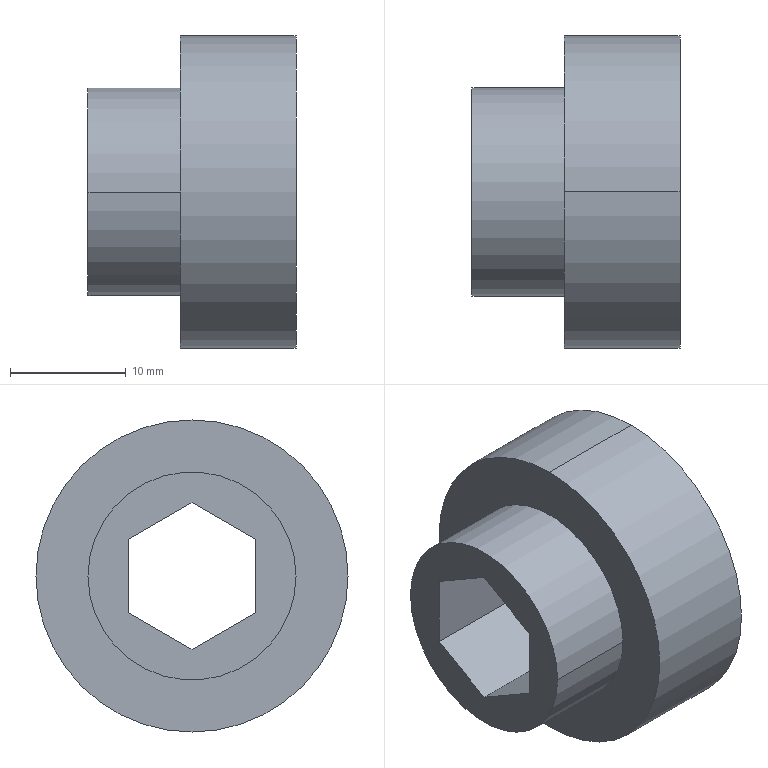Part | NX | features BREP 1 | 1 solid | 13 faces | box 18 x 27 x 27 mm | volume 5875 mm3 | plane 9 | cylinder 4 | commonest cylinder face diameters 18 x2 27 x2
STEP:
#1=CARTESIAN_POINT('',(-5.,0.,13.5));
#2=VERTEX_POINT('',#1);
#3=CARTESIAN_POINT('',(-5.,0.,-13.5));
#4=VERTEX_POINT('',#3);
#5=CARTESIAN_POINT('',(-5.,0.,0.));
#6=DIRECTION('',(1.,0.,0.));
#7=DIRECTION('',(0.,0.,1.));
#8=AXIS2_PLACEMENT_3D('',#5,#6,#7);
#9=CIRCLE('',#8,13.5);
#10=EDGE_CURVE('',#2,#4,#9,.T.);
#11=ORIENTED_EDGE('',*,*,#10,.F.);
#12=CARTESIAN_POINT('',(-5.,0.,0.));
#13=DIRECTION('',(1.,0.,0.));
#14=DIRECTION('',(0.,0.,-1.));
#15=AXIS2_PLACEMENT_3D('',#12,#13,#14);
#16=CIRCLE('',#15,13.5);
#17=EDGE_CURVE('',#4,#2,#16,.T.);
#18=ORIENTED_EDGE('',*,*,#17,.F.);
#19=EDGE_LOOP('',(#11,#18));
#20=FACE_BOUND('',#19,.T.);
#21=CARTESIAN_POINT('',(-5.,-9.,0.));
#22=VERTEX_POINT('',#21);
#23=CARTESIAN_POINT('',(-5.,9.,0.));
#24=VERTEX_POINT('',#23);
#25=CARTESIAN_POINT('',(-5.,0.,0.));
#26=DIRECTION('',(-1.,0.,0.));
#27=DIRECTION('',(0.,-1.,0.));
#28=AXIS2_PLACEMENT_3D('',#25,#26,#27);
#29=CIRCLE('',#28,9.);
#30=EDGE_CURVE('',#22,#24,#29,.T.);
#31=ORIENTED_EDGE('',*,*,#30,.F.);
#32=CARTESIAN_POINT('',(-5.,0.,0.));
#33=DIRECTION('',(-1.,0.,0.));
#34=DIRECTION('',(0.,1.,0.));
#35=AXIS2_PLACEMENT_3D('',#32,#33,#34);
#36=CIRCLE('',#35,9.);
#37=EDGE_CURVE('',#24,#22,#36,.T.);
#38=ORIENTED_EDGE('',*,*,#37,.F.);
#39=EDGE_LOOP('',(#31,#38));
#40=FACE_BOUND('',#39,.T.);
#41=CARTESIAN_POINT('',(-5.,0.,0.));
#42=DIRECTION('',(1.,0.,0.));
#43=DIRECTION('',(0.,1.,0.));
#44=AXIS2_PLACEMENT_3D('',#41,#42,#43);
#45=PLANE('',#44);
#46=ADVANCED_FACE('',(#20,#40),#45,.F.);
#47=CARTESIAN_POINT('',(5.,0.,13.5));
#48=VERTEX_POINT('',#47);
#49=CARTESIAN_POINT('',(-5.,0.,13.5));
#50=DIRECTION('',(1.,0.,0.));
#51=VECTOR('',#50,1000.);
#52=LINE('',#49,#51);
#53=EDGE_CURVE('',#48,#2,#52,.F.);
#54=ORIENTED_EDGE('',*,*,#53,.F.);
#55=CARTESIAN_POINT('',(5.,0.,-13.5));
#56=VERTEX_POINT('',#55);
#57=CARTESIAN_POINT('',(5.,0.,0.));
#58=DIRECTION('',(1.,0.,0.));
#59=DIRECTION('',(0.,0.,-1.));
#60=AXIS2_PLACEMENT_3D('',#57,#58,#59);
#61=CIRCLE('',#60,13.5);
#62=EDGE_CURVE('',#56,#48,#61,.T.);
#63=ORIENTED_EDGE('',*,*,#62,.F.);
#64=CARTESIAN_POINT('',(-5.,0.,-13.5));
#65=DIRECTION('',(1.,0.,0.));
#66=VECTOR('',#65,1000.);
#67=LINE('',#64,#66);
#68=EDGE_CURVE('',#56,#4,#67,.F.);
#69=ORIENTED_EDGE('',*,*,#68,.T.);
#70=ORIENTED_EDGE('',*,*,#17,.T.);
#71=EDGE_LOOP('',(#54,#63,#69,#70));
#72=FACE_BOUND('',#71,.T.);
#73=CARTESIAN_POINT('',(-5.,0.,0.));
#74=DIRECTION('',(1.,0.,0.));
#75=DIRECTION('',(0.,0.,-1.));
#76=AXIS2_PLACEMENT_3D('',#73,#74,#75);
#77=CYLINDRICAL_SURFACE('',#76,13.5);
#78=ADVANCED_FACE('',(#72),#77,.T.);
#79=ORIENTED_EDGE('',*,*,#68,.F.);
#80=CARTESIAN_POINT('',(5.,0.,0.));
#81=DIRECTION('',(1.,0.,0.));
#82=DIRECTION('',(0.,0.,1.));
#83=AXIS2_PLACEMENT_3D('',#80,#81,#82);
#84=CIRCLE('',#83,13.5);
#85=EDGE_CURVE('',#48,#56,#84,.T.);
#86=ORIENTED_EDGE('',*,*,#85,.F.);
#87=ORIENTED_EDGE('',*,*,#53,.T.);
#88=ORIENTED_EDGE('',*,*,#10,.T.);
#89=EDGE_LOOP('',(#79,#86,#87,#88));
#90=FACE_BOUND('',#89,.T.);
#91=CARTESIAN_POINT('',(-5.,0.,0.));
#92=DIRECTION('',(1.,0.,0.));
#93=DIRECTION('',(0.,0.,-1.));
#94=AXIS2_PLACEMENT_3D('',#91,#92,#93);
#95=CYLINDRICAL_SURFACE('',#94,13.5);
#96=ADVANCED_FACE('',(#90),#95,.T.);
#97=ORIENTED_EDGE('',*,*,#85,.T.);
#98=ORIENTED_EDGE('',*,*,#62,.T.);
#99=EDGE_LOOP('',(#97,#98));
#100=FACE_BOUND('',#99,.T.);
#101=CARTESIAN_POINT('',(5.,5.5,-3.175));
#102=VERTEX_POINT('',#101);
#103=CARTESIAN_POINT('',(5.,5.5,3.175));
#104=VERTEX_POINT('',#103);
#105=CARTESIAN_POINT('',(5.,5.5,-3.175));
#106=DIRECTION('',(0.,0.,1.));
#107=VECTOR('',#106,1000.);
#108=LINE('',#105,#107);
#109=EDGE_CURVE('',#102,#104,#108,.T.);
#110=ORIENTED_EDGE('',*,*,#109,.F.);
#111=CARTESIAN_POINT('',(5.,0.,-6.351));
#112=VERTEX_POINT('',#111);
#113=CARTESIAN_POINT('',(5.,0.,-6.351));
#114=DIRECTION('',(0.,0.866,0.5));
#115=VECTOR('',#114,1000.);
#116=LINE('',#113,#115);
#117=EDGE_CURVE('',#112,#102,#116,.T.);
#118=ORIENTED_EDGE('',*,*,#117,.F.);
#119=CARTESIAN_POINT('',(5.,-5.5,-3.175));
#120=VERTEX_POINT('',#119);
#121=CARTESIAN_POINT('',(5.,-5.5,-3.175));
#122=DIRECTION('',(0.,0.866,-0.5));
#123=VECTOR('',#122,1000.);
#124=LINE('',#121,#123);
#125=EDGE_CURVE('',#120,#112,#124,.T.);
#126=ORIENTED_EDGE('',*,*,#125,.F.);
#127=CARTESIAN_POINT('',(5.,-5.5,3.175));
#128=VERTEX_POINT('',#127);
#129=CARTESIAN_POINT('',(5.,-5.5,3.175));
#130=DIRECTION('',(0.,0.,-1.));
#131=VECTOR('',#130,1000.);
#132=LINE('',#129,#131);
#133=EDGE_CURVE('',#128,#120,#132,.T.);
#134=ORIENTED_EDGE('',*,*,#133,.F.);
#135=CARTESIAN_POINT('',(5.,0.,6.351));
#136=VERTEX_POINT('',#135);
#137=CARTESIAN_POINT('',(5.,0.,6.351));
#138=DIRECTION('',(0.,-0.866,-0.5));
#139=VECTOR('',#138,1000.);
#140=LINE('',#137,#139);
#141=EDGE_CURVE('',#136,#128,#140,.T.);
#142=ORIENTED_EDGE('',*,*,#141,.F.);
#143=CARTESIAN_POINT('',(5.,5.5,3.175));
#144=DIRECTION('',(0.,-0.866,0.5));
#145=VECTOR('',#144,1000.);
#146=LINE('',#143,#145);
#147=EDGE_CURVE('',#104,#136,#146,.T.);
#148=ORIENTED_EDGE('',*,*,#147,.F.);
#149=EDGE_LOOP('',(#110,#118,#126,#134,#142,#148));
#150=FACE_BOUND('',#149,.T.);
#151=CARTESIAN_POINT('',(5.,0.,0.));
#152=DIRECTION('',(1.,0.,0.));
#153=DIRECTION('',(0.,1.,0.));
#154=AXIS2_PLACEMENT_3D('',#151,#152,#153);
#155=PLANE('',#154);
#156=ADVANCED_FACE('',(#100,#150),#155,.T.);
#157=CARTESIAN_POINT('',(-13.,0.,6.351));
#158=VERTEX_POINT('',#157);
#159=CARTESIAN_POINT('',(5.,0.,6.351));
#160=DIRECTION('',(-1.,0.,0.));
#161=VECTOR('',#160,1000.);
#162=LINE('',#159,#161);
#163=EDGE_CURVE('',#136,#158,#162,.T.);
#164=ORIENTED_EDGE('',*,*,#163,.T.);
#165=CARTESIAN_POINT('',(-13.,5.5,3.175));
#166=VERTEX_POINT('',#165);
#167=CARTESIAN_POINT('',(-13.,5.5,3.175));
#168=DIRECTION('',(0.,-0.866,0.5));
#169=VECTOR('',#168,1000.);
#170=LINE('',#167,#169);
#171=EDGE_CURVE('',#166,#158,#170,.T.);
#172=ORIENTED_EDGE('',*,*,#171,.F.);
#173=CARTESIAN_POINT('',(5.,5.5,3.175));
#174=DIRECTION('',(-1.,0.,0.));
#175=VECTOR('',#174,1000.);
#176=LINE('',#173,#175);
#177=EDGE_CURVE('',#104,#166,#176,.T.);
#178=ORIENTED_EDGE('',*,*,#177,.F.);
#179=ORIENTED_EDGE('',*,*,#147,.T.);
#180=EDGE_LOOP('',(#164,#172,#178,#179));
#181=FACE_BOUND('',#180,.T.);
#182=CARTESIAN_POINT('',(6.8,5.5,3.175));
#183=DIRECTION('',(0.,0.5,0.866));
#184=DIRECTION('',(1.,0.,0.));
#185=AXIS2_PLACEMENT_3D('',#182,#183,#184);
#186=PLANE('',#185);
#187=ADVANCED_FACE('',(#181),#186,.F.);
#188=ORIENTED_EDGE('',*,*,#177,.T.);
#189=CARTESIAN_POINT('',(-13.,5.5,-3.175));
#190=VERTEX_POINT('',#189);
#191=CARTESIAN_POINT('',(-13.,5.5,-3.175));
#192=DIRECTION('',(0.,0.,1.));
#193=VECTOR('',#192,1000.);
#194=LINE('',#191,#193);
#195=EDGE_CURVE('',#190,#166,#194,.T.);
#196=ORIENTED_EDGE('',*,*,#195,.F.);
#197=CARTESIAN_POINT('',(5.,5.5,-3.175));
#198=DIRECTION('',(-1.,0.,0.));
#199=VECTOR('',#198,1000.);
#200=LINE('',#197,#199);
#201=EDGE_CURVE('',#102,#190,#200,.T.);
#202=ORIENTED_EDGE('',*,*,#201,.F.);
#203=ORIENTED_EDGE('',*,*,#109,.T.);
#204=EDGE_LOOP('',(#188,#196,#202,#203));
#205=FACE_BOUND('',#204,.T.);
#206=CARTESIAN_POINT('',(6.8,5.5,-3.175));
#207=DIRECTION('',(0.,1.,0.));
#208=DIRECTION('',(1.,0.,0.));
#209=AXIS2_PLACEMENT_3D('',#206,#207,#208);
#210=PLANE('',#209);
#211=ADVANCED_FACE('',(#205),#210,.F.);
#212=ORIENTED_EDGE('',*,*,#201,.T.);
#213=CARTESIAN_POINT('',(-13.,0.,-6.351));
#214=VERTEX_POINT('',#213);
#215=CARTESIAN_POINT('',(-13.,0.,-6.351));
#216=DIRECTION('',(0.,0.866,0.5));
#217=VECTOR('',#216,1000.);
#218=LINE('',#215,#217);
#219=EDGE_CURVE('',#214,#190,#218,.T.);
#220=ORIENTED_EDGE('',*,*,#219,.F.);
#221=CARTESIAN_POINT('',(5.,0.,-6.351));
#222=DIRECTION('',(-1.,0.,0.));
#223=VECTOR('',#222,1000.);
#224=LINE('',#221,#223);
#225=EDGE_CURVE('',#112,#214,#224,.T.);
#226=ORIENTED_EDGE('',*,*,#225,.F.);
#227=ORIENTED_EDGE('',*,*,#117,.T.);
#228=EDGE_LOOP('',(#212,#220,#226,#227));
#229=FACE_BOUND('',#228,.T.);
#230=CARTESIAN_POINT('',(6.8,0.,-6.351));
#231=DIRECTION('',(0.,0.5,-0.866));
#232=DIRECTION('',(-1.,0.,0.));
#233=AXIS2_PLACEMENT_3D('',#230,#231,#232);
#234=PLANE('',#233);
#235=ADVANCED_FACE('',(#229),#234,.F.);
#236=ORIENTED_EDGE('',*,*,#225,.T.);
#237=CARTESIAN_POINT('',(-13.,-5.5,-3.175));
#238=VERTEX_POINT('',#237);
#239=CARTESIAN_POINT('',(-13.,-5.5,-3.175));
#240=DIRECTION('',(0.,0.866,-0.5));
#241=VECTOR('',#240,1000.);
#242=LINE('',#239,#241);
#243=EDGE_CURVE('',#238,#214,#242,.T.);
#244=ORIENTED_EDGE('',*,*,#243,.F.);
#245=CARTESIAN_POINT('',(5.,-5.5,-3.175));
#246=DIRECTION('',(-1.,0.,0.));
#247=VECTOR('',#246,1000.);
#248=LINE('',#245,#247);
#249=EDGE_CURVE('',#120,#238,#248,.T.);
#250=ORIENTED_EDGE('',*,*,#249,.F.);
#251=ORIENTED_EDGE('',*,*,#125,.T.);
#252=EDGE_LOOP('',(#236,#244,#250,#251));
#253=FACE_BOUND('',#252,.T.);
#254=CARTESIAN_POINT('',(6.8,-5.5,-3.175));
#255=DIRECTION('',(0.,-0.5,-0.866));
#256=DIRECTION('',(0.,-0.866,0.5));
#257=AXIS2_PLACEMENT_3D('',#254,#255,#256);
#258=PLANE('',#257);
#259=ADVANCED_FACE('',(#253),#258,.F.);
#260=ORIENTED_EDGE('',*,*,#249,.T.);
#261=CARTESIAN_POINT('',(-13.,-5.5,3.175));
#262=VERTEX_POINT('',#261);
#263=CARTESIAN_POINT('',(-13.,-5.5,3.175));
#264=DIRECTION('',(0.,0.,-1.));
#265=VECTOR('',#264,1000.);
#266=LINE('',#263,#265);
#267=EDGE_CURVE('',#262,#238,#266,.T.);
#268=ORIENTED_EDGE('',*,*,#267,.F.);
#269=CARTESIAN_POINT('',(5.,-5.5,3.175));
#270=DIRECTION('',(-1.,0.,0.));
#271=VECTOR('',#270,1000.);
#272=LINE('',#269,#271);
#273=EDGE_CURVE('',#128,#262,#272,.T.);
#274=ORIENTED_EDGE('',*,*,#273,.F.);
#275=ORIENTED_EDGE('',*,*,#133,.T.);
#276=EDGE_LOOP('',(#260,#268,#274,#275));
#277=FACE_BOUND('',#276,.T.);
#278=CARTESIAN_POINT('',(6.8,-5.5,3.175));
#279=DIRECTION('',(0.,-1.,0.));
#280=DIRECTION('',(0.,0.,-1.));
#281=AXIS2_PLACEMENT_3D('',#278,#279,#280);
#282=PLANE('',#281);
#283=ADVANCED_FACE('',(#277),#282,.F.);
#284=ORIENTED_EDGE('',*,*,#273,.T.);
#285=CARTESIAN_POINT('',(-13.,0.,6.351));
#286=DIRECTION('',(0.,-0.866,-0.5));
#287=VECTOR('',#286,1000.);
#288=LINE('',#285,#287);
#289=EDGE_CURVE('',#158,#262,#288,.T.);
#290=ORIENTED_EDGE('',*,*,#289,.F.);
#291=ORIENTED_EDGE('',*,*,#163,.F.);
#292=ORIENTED_EDGE('',*,*,#141,.T.);
#293=EDGE_LOOP('',(#284,#290,#291,#292));
#294=FACE_BOUND('',#293,.T.);
#295=CARTESIAN_POINT('',(6.8,0.,6.351));
#296=DIRECTION('',(0.,-0.5,0.866));
#297=DIRECTION('',(-1.,0.,0.));
#298=AXIS2_PLACEMENT_3D('',#295,#296,#297);
#299=PLANE('',#298);
#300=ADVANCED_FACE('',(#294),#299,.F.);
#301=CARTESIAN_POINT('',(-13.,-9.,0.));
#302=VERTEX_POINT('',#301);
#303=CARTESIAN_POINT('',(-13.,9.,0.));
#304=VERTEX_POINT('',#303);
#305=CARTESIAN_POINT('',(-13.,0.,0.));
#306=DIRECTION('',(-1.,0.,0.));
#307=DIRECTION('',(0.,-1.,0.));
#308=AXIS2_PLACEMENT_3D('',#305,#306,#307);
#309=CIRCLE('',#308,9.);
#310=EDGE_CURVE('',#302,#304,#309,.T.);
#311=ORIENTED_EDGE('',*,*,#310,.T.);
#312=CARTESIAN_POINT('',(-13.,0.,0.));
#313=DIRECTION('',(-1.,0.,0.));
#314=DIRECTION('',(0.,1.,0.));
#315=AXIS2_PLACEMENT_3D('',#312,#313,#314);
#316=CIRCLE('',#315,9.);
#317=EDGE_CURVE('',#304,#302,#316,.T.);
#318=ORIENTED_EDGE('',*,*,#317,.T.);
#319=EDGE_LOOP('',(#311,#318));
#320=FACE_BOUND('',#319,.T.);
#321=ORIENTED_EDGE('',*,*,#289,.T.);
#322=ORIENTED_EDGE('',*,*,#267,.T.);
#323=ORIENTED_EDGE('',*,*,#243,.T.);
#324=ORIENTED_EDGE('',*,*,#219,.T.);
#325=ORIENTED_EDGE('',*,*,#195,.T.);
#326=ORIENTED_EDGE('',*,*,#171,.T.);
#327=EDGE_LOOP('',(#321,#322,#323,#324,#325,#326));
#328=FACE_BOUND('',#327,.T.);
#329=CARTESIAN_POINT('',(-13.,0.,0.));
#330=DIRECTION('',(-1.,0.,0.));
#331=DIRECTION('',(0.,0.,1.));
#332=AXIS2_PLACEMENT_3D('',#329,#330,#331);
#333=PLANE('',#332);
#334=ADVANCED_FACE('',(#320,#328),#333,.T.);
#335=CARTESIAN_POINT('',(-5.,-9.,0.));
#336=DIRECTION('',(-1.,0.,0.));
#337=VECTOR('',#336,1000.);
#338=LINE('',#335,#337);
#339=EDGE_CURVE('',#22,#302,#338,.T.);
#340=ORIENTED_EDGE('',*,*,#339,.T.);
#341=ORIENTED_EDGE('',*,*,#317,.F.);
#342=CARTESIAN_POINT('',(-5.,9.,0.));
#343=DIRECTION('',(-1.,0.,0.));
#344=VECTOR('',#343,1000.);
#345=LINE('',#342,#344);
#346=EDGE_CURVE('',#24,#304,#345,.T.);
#347=ORIENTED_EDGE('',*,*,#346,.F.);
#348=ORIENTED_EDGE('',*,*,#37,.T.);
#349=EDGE_LOOP('',(#340,#341,#347,#348));
#350=FACE_BOUND('',#349,.T.);
#351=CARTESIAN_POINT('',(-5.,0.,0.));
#352=DIRECTION('',(-1.,0.,0.));
#353=DIRECTION('',(0.,1.,0.));
#354=AXIS2_PLACEMENT_3D('',#351,#352,#353);
#355=CYLINDRICAL_SURFACE('',#354,9.);
#356=ADVANCED_FACE('',(#350),#355,.T.);
#357=ORIENTED_EDGE('',*,*,#346,.T.);
#358=ORIENTED_EDGE('',*,*,#310,.F.);
#359=ORIENTED_EDGE('',*,*,#339,.F.);
#360=ORIENTED_EDGE('',*,*,#30,.T.);
#361=EDGE_LOOP('',(#357,#358,#359,#360));
#362=FACE_BOUND('',#361,.T.);
#363=CARTESIAN_POINT('',(-5.,0.,0.));
#364=DIRECTION('',(-1.,0.,0.));
#365=DIRECTION('',(0.,1.,0.));
#366=AXIS2_PLACEMENT_3D('',#363,#364,#365);
#367=CYLINDRICAL_SURFACE('',#366,9.);
#368=ADVANCED_FACE('',(#362),#367,.T.);
#369=CLOSED_SHELL('',(#46,#78,#96,#156,#187,#211,#235,#259,#283,#300,#334,#356,#368));
#370=MANIFOLD_SOLID_BREP('',#369);
#371=(LENGTH_UNIT()NAMED_UNIT(*)SI_UNIT(.MILLI.,.METRE.));
#372=UNCERTAINTY_MEASURE_WITH_UNIT(LENGTH_MEASURE(0.00001),#371,'','');
#373=(NAMED_UNIT(*)PLANE_ANGLE_UNIT()SI_UNIT($,.RADIAN.));
#374=(NAMED_UNIT(*)SI_UNIT($,.STERADIAN.)SOLID_ANGLE_UNIT());
#375=(GEOMETRIC_REPRESENTATION_CONTEXT(3)GLOBAL_UNCERTAINTY_ASSIGNED_CONTEXT((#372))GLOBAL_UNIT_ASSIGNED_CONTEXT((#371,#373,#374))REPRESENTATION_CONTEXT('',''));
#376=ADVANCED_BREP_SHAPE_REPRESENTATION('',(#370),#375);